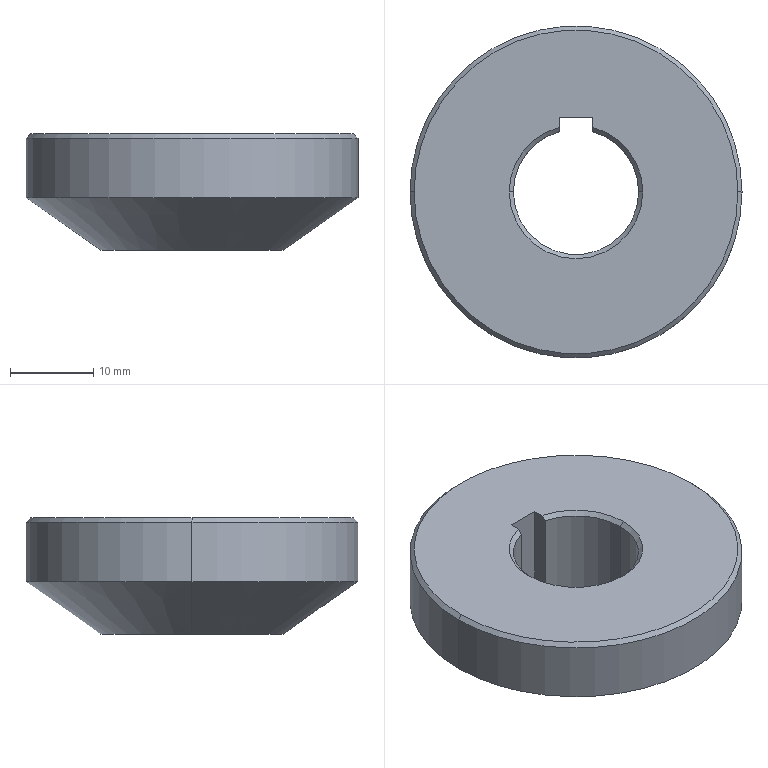Part | STEP file | 10000020570swp000-1 | 1 solid | 20 faces | box 40 x 40 x 14 mm | volume 11944 mm3 | cone 10 | cylinder 5 | plane 5 | commonest cylinder face diameters 15.1 x3 40 x2
STEP:
#1=CARTESIAN_POINT('',(-7.55,0.,-0.5));
#2=VERTEX_POINT('',#1);
#3=CARTESIAN_POINT('',(7.55,0.,-0.5));
#4=VERTEX_POINT('',#3);
#5=CARTESIAN_POINT('',(0.,0.,-0.5));
#6=DIRECTION('',(0.,0.,1.));
#7=DIRECTION('',(1.,0.,0.));
#8=AXIS2_PLACEMENT_3D('',#5,#6,#7);
#9=CIRCLE('',#8,7.55);
#10=EDGE_CURVE('',#2,#4,#9,.T.);
#11=ORIENTED_EDGE('',*,*,#10,.F.);
#12=CARTESIAN_POINT('',(-8.05,0.,0.));
#13=VERTEX_POINT('',#12);
#14=CARTESIAN_POINT('',(-7.55,0.,-0.5));
#15=DIRECTION('',(-0.7071,0.,0.7071));
#16=VECTOR('',#15,1000.);
#17=LINE('',#14,#16);
#18=EDGE_CURVE('',#2,#13,#17,.T.);
#19=ORIENTED_EDGE('',*,*,#18,.T.);
#20=CARTESIAN_POINT('',(8.05,0.,0.));
#21=VERTEX_POINT('',#20);
#22=CARTESIAN_POINT('',(0.,0.,0.));
#23=DIRECTION('',(0.,0.,-1.));
#24=DIRECTION('',(1.,0.,0.));
#25=AXIS2_PLACEMENT_3D('',#22,#23,#24);
#26=CIRCLE('',#25,8.05);
#27=EDGE_CURVE('',#21,#13,#26,.T.);
#28=ORIENTED_EDGE('',*,*,#27,.F.);
#29=CARTESIAN_POINT('',(7.55,0.,-0.5));
#30=DIRECTION('',(0.7071,0.,0.7071));
#31=VECTOR('',#30,1000.);
#32=LINE('',#29,#31);
#33=EDGE_CURVE('',#4,#21,#32,.T.);
#34=ORIENTED_EDGE('',*,*,#33,.F.);
#35=EDGE_LOOP('',(#11,#19,#28,#34));
#36=FACE_OUTER_BOUND('',#35,.T.);
#37=CARTESIAN_POINT('',(0.,0.,-0.5));
#38=DIRECTION('',(0.,0.,1.));
#39=DIRECTION('',(1.,0.,0.));
#40=AXIS2_PLACEMENT_3D('',#37,#38,#39);
#41=CONICAL_SURFACE('',#40,7.55,0.7854);
#42=ADVANCED_FACE('',(#36),#41,.F.);
#43=CARTESIAN_POINT('',(2.,7.28,-0.5));
#44=VERTEX_POINT('',#43);
#45=CARTESIAN_POINT('',(0.,0.,-0.5));
#46=DIRECTION('',(0.,0.,1.));
#47=DIRECTION('',(1.,0.,0.));
#48=AXIS2_PLACEMENT_3D('',#45,#46,#47);
#49=CIRCLE('',#48,7.55);
#50=EDGE_CURVE('',#4,#44,#49,.T.);
#51=ORIENTED_EDGE('',*,*,#50,.F.);
#52=ORIENTED_EDGE('',*,*,#33,.T.);
#53=CARTESIAN_POINT('',(2.,7.798,0.));
#54=VERTEX_POINT('',#53);
#55=CARTESIAN_POINT('',(0.,0.,0.));
#56=DIRECTION('',(0.,0.,-1.));
#57=DIRECTION('',(1.,0.,0.));
#58=AXIS2_PLACEMENT_3D('',#55,#56,#57);
#59=CIRCLE('',#58,8.05);
#60=EDGE_CURVE('',#54,#21,#59,.T.);
#61=ORIENTED_EDGE('',*,*,#60,.F.);
#62=CARTESIAN_POINT('',(2.,7.28,-0.5));
#63=CARTESIAN_POINT('',(2.,7.453,-0.3335));
#64=CARTESIAN_POINT('',(2.,7.625,-0.1669));
#65=CARTESIAN_POINT('',(2.,7.798,0.));
#66=B_SPLINE_CURVE_WITH_KNOTS('',3,(#62,#63,#64,#65),.UNSPECIFIED.,.F.,.F.,(4,4),(0.,0.0007195),.UNSPECIFIED.);
#67=EDGE_CURVE('',#44,#54,#66,.T.);
#68=ORIENTED_EDGE('',*,*,#67,.F.);
#69=EDGE_LOOP('',(#51,#52,#61,#68));
#70=FACE_OUTER_BOUND('',#69,.T.);
#71=CARTESIAN_POINT('',(0.,0.,-0.5));
#72=DIRECTION('',(0.,0.,1.));
#73=DIRECTION('',(1.,0.,0.));
#74=AXIS2_PLACEMENT_3D('',#71,#72,#73);
#75=CONICAL_SURFACE('',#74,7.55,0.7854);
#76=ADVANCED_FACE('',(#70),#75,.F.);
#77=CARTESIAN_POINT('',(7.55,0.,-13.5));
#78=VERTEX_POINT('',#77);
#79=CARTESIAN_POINT('',(-7.55,0.,-13.5));
#80=VERTEX_POINT('',#79);
#81=CARTESIAN_POINT('',(0.,0.,-13.5));
#82=DIRECTION('',(0.,0.,-1.));
#83=DIRECTION('',(1.,0.,0.));
#84=AXIS2_PLACEMENT_3D('',#81,#82,#83);
#85=CIRCLE('',#84,7.55);
#86=EDGE_CURVE('',#78,#80,#85,.T.);
#87=ORIENTED_EDGE('',*,*,#86,.F.);
#88=CARTESIAN_POINT('',(8.05,0.,-14.));
#89=VERTEX_POINT('',#88);
#90=CARTESIAN_POINT('',(8.05,0.,-14.));
#91=DIRECTION('',(0.7071,0.,-0.7071));
#92=VECTOR('',#91,1000.);
#93=LINE('',#90,#92);
#94=EDGE_CURVE('',#78,#89,#93,.T.);
#95=ORIENTED_EDGE('',*,*,#94,.T.);
#96=CARTESIAN_POINT('',(-8.05,0.,-14.));
#97=VERTEX_POINT('',#96);
#98=CARTESIAN_POINT('',(0.,0.,-14.));
#99=DIRECTION('',(0.,0.,1.));
#100=DIRECTION('',(1.,0.,0.));
#101=AXIS2_PLACEMENT_3D('',#98,#99,#100);
#102=CIRCLE('',#101,8.05);
#103=EDGE_CURVE('',#97,#89,#102,.T.);
#104=ORIENTED_EDGE('',*,*,#103,.F.);
#105=CARTESIAN_POINT('',(-8.05,0.,-14.));
#106=DIRECTION('',(-0.7071,0.,-0.7071));
#107=VECTOR('',#106,1000.);
#108=LINE('',#105,#107);
#109=EDGE_CURVE('',#80,#97,#108,.T.);
#110=ORIENTED_EDGE('',*,*,#109,.F.);
#111=EDGE_LOOP('',(#87,#95,#104,#110));
#112=FACE_OUTER_BOUND('',#111,.T.);
#113=CARTESIAN_POINT('',(0.,0.,-14.));
#114=DIRECTION('',(0.,0.,-1.));
#115=DIRECTION('',(-1.,0.,0.));
#116=AXIS2_PLACEMENT_3D('',#113,#114,#115);
#117=CONICAL_SURFACE('',#116,8.05,0.7854);
#118=ADVANCED_FACE('',(#112),#117,.F.);
#119=CARTESIAN_POINT('',(-2.,7.28,-13.5));
#120=VERTEX_POINT('',#119);
#121=CARTESIAN_POINT('',(0.,0.,-13.5));
#122=DIRECTION('',(0.,0.,-1.));
#123=DIRECTION('',(1.,0.,0.));
#124=AXIS2_PLACEMENT_3D('',#121,#122,#123);
#125=CIRCLE('',#124,7.55);
#126=EDGE_CURVE('',#80,#120,#125,.T.);
#127=ORIENTED_EDGE('',*,*,#126,.F.);
#128=ORIENTED_EDGE('',*,*,#109,.T.);
#129=CARTESIAN_POINT('',(-2.,7.798,-14.));
#130=VERTEX_POINT('',#129);
#131=CARTESIAN_POINT('',(0.,0.,-14.));
#132=DIRECTION('',(0.,0.,1.));
#133=DIRECTION('',(1.,0.,0.));
#134=AXIS2_PLACEMENT_3D('',#131,#132,#133);
#135=CIRCLE('',#134,8.05);
#136=EDGE_CURVE('',#130,#97,#135,.T.);
#137=ORIENTED_EDGE('',*,*,#136,.F.);
#138=CARTESIAN_POINT('',(-2.,7.28,-13.5));
#139=CARTESIAN_POINT('',(-2.,7.453,-13.666));
#140=CARTESIAN_POINT('',(-2.,7.625,-13.833));
#141=CARTESIAN_POINT('',(-2.,7.798,-14.));
#142=B_SPLINE_CURVE_WITH_KNOTS('',3,(#138,#139,#140,#141),.UNSPECIFIED.,.F.,.F.,(4,4),(0.,0.0007195),.UNSPECIFIED.);
#143=EDGE_CURVE('',#120,#130,#142,.T.);
#144=ORIENTED_EDGE('',*,*,#143,.F.);
#145=EDGE_LOOP('',(#127,#128,#137,#144));
#146=FACE_OUTER_BOUND('',#145,.T.);
#147=CARTESIAN_POINT('',(0.,0.,-14.));
#148=DIRECTION('',(0.,0.,-1.));
#149=DIRECTION('',(-1.,0.,0.));
#150=AXIS2_PLACEMENT_3D('',#147,#148,#149);
#151=CONICAL_SURFACE('',#150,8.05,0.7854);
#152=ADVANCED_FACE('',(#146),#151,.F.);
#153=CARTESIAN_POINT('',(19.5,0.,0.));
#154=VERTEX_POINT('',#153);
#155=CARTESIAN_POINT('',(-19.5,0.,0.));
#156=VERTEX_POINT('',#155);
#157=CARTESIAN_POINT('',(0.,0.,0.));
#158=DIRECTION('',(0.,0.,1.));
#159=DIRECTION('',(1.,0.,0.));
#160=AXIS2_PLACEMENT_3D('',#157,#158,#159);
#161=CIRCLE('',#160,19.5);
#162=EDGE_CURVE('',#154,#156,#161,.T.);
#163=ORIENTED_EDGE('',*,*,#162,.F.);
#164=CARTESIAN_POINT('',(20.,0.,-0.5));
#165=VERTEX_POINT('',#164);
#166=CARTESIAN_POINT('',(19.5,0.,0.));
#167=DIRECTION('',(0.7071,0.,-0.7071));
#168=VECTOR('',#167,1000.);
#169=LINE('',#166,#168);
#170=EDGE_CURVE('',#154,#165,#169,.T.);
#171=ORIENTED_EDGE('',*,*,#170,.T.);
#172=CARTESIAN_POINT('',(-20.,0.,-0.5));
#173=VERTEX_POINT('',#172);
#174=CARTESIAN_POINT('',(0.,0.,-0.5));
#175=DIRECTION('',(0.,0.,-1.));
#176=DIRECTION('',(1.,0.,0.));
#177=AXIS2_PLACEMENT_3D('',#174,#175,#176);
#178=CIRCLE('',#177,20.);
#179=EDGE_CURVE('',#173,#165,#178,.T.);
#180=ORIENTED_EDGE('',*,*,#179,.F.);
#181=CARTESIAN_POINT('',(-19.5,0.,0.));
#182=DIRECTION('',(-0.7071,0.,-0.7071));
#183=VECTOR('',#182,1000.);
#184=LINE('',#181,#183);
#185=EDGE_CURVE('',#156,#173,#184,.T.);
#186=ORIENTED_EDGE('',*,*,#185,.F.);
#187=EDGE_LOOP('',(#163,#171,#180,#186));
#188=FACE_OUTER_BOUND('',#187,.T.);
#189=CARTESIAN_POINT('',(0.,0.,0.));
#190=DIRECTION('',(0.,0.,-1.));
#191=DIRECTION('',(-1.,0.,0.));
#192=AXIS2_PLACEMENT_3D('',#189,#190,#191);
#193=CONICAL_SURFACE('',#192,19.5,0.7854);
#194=ADVANCED_FACE('',(#188),#193,.T.);
#195=CARTESIAN_POINT('',(11.,0.,-14.));
#196=VERTEX_POINT('',#195);
#197=CARTESIAN_POINT('',(-11.,0.,-14.));
#198=VERTEX_POINT('',#197);
#199=CARTESIAN_POINT('',(0.,0.,-14.));
#200=DIRECTION('',(0.,0.,1.));
#201=DIRECTION('',(1.,0.,0.));
#202=AXIS2_PLACEMENT_3D('',#199,#200,#201);
#203=CIRCLE('',#202,11.);
#204=EDGE_CURVE('',#196,#198,#203,.T.);
#205=ORIENTED_EDGE('',*,*,#204,.T.);
#206=CARTESIAN_POINT('',(-20.,0.,-7.698));
#207=VERTEX_POINT('',#206);
#208=CARTESIAN_POINT('',(-11.,0.,-14.));
#209=DIRECTION('',(-0.8192,0.,0.5736));
#210=VECTOR('',#209,1000.);
#211=LINE('',#208,#210);
#212=EDGE_CURVE('',#198,#207,#211,.T.);
#213=ORIENTED_EDGE('',*,*,#212,.T.);
#214=CARTESIAN_POINT('',(20.,0.,-7.698));
#215=VERTEX_POINT('',#214);
#216=CARTESIAN_POINT('',(0.,0.,-7.698));
#217=DIRECTION('',(0.,0.,1.));
#218=DIRECTION('',(1.,0.,0.));
#219=AXIS2_PLACEMENT_3D('',#216,#217,#218);
#220=CIRCLE('',#219,20.);
#221=EDGE_CURVE('',#215,#207,#220,.T.);
#222=ORIENTED_EDGE('',*,*,#221,.F.);
#223=CARTESIAN_POINT('',(11.,0.,-14.));
#224=DIRECTION('',(0.8192,0.,0.5736));
#225=VECTOR('',#224,1000.);
#226=LINE('',#223,#225);
#227=EDGE_CURVE('',#196,#215,#226,.T.);
#228=ORIENTED_EDGE('',*,*,#227,.F.);
#229=EDGE_LOOP('',(#205,#213,#222,#228));
#230=FACE_OUTER_BOUND('',#229,.T.);
#231=CARTESIAN_POINT('',(0.,0.,-14.));
#232=DIRECTION('',(0.,0.,1.));
#233=DIRECTION('',(1.,0.,0.));
#234=AXIS2_PLACEMENT_3D('',#231,#232,#233);
#235=CONICAL_SURFACE('',#234,11.,0.9599);
#236=ADVANCED_FACE('',(#230),#235,.T.);
#237=ORIENTED_EDGE('',*,*,#86,.T.);
#238=CARTESIAN_POINT('',(-7.55,0.,-14.));
#239=DIRECTION('',(0.,0.,1.));
#240=VECTOR('',#239,1000.);
#241=LINE('',#238,#240);
#242=EDGE_CURVE('',#80,#2,#241,.T.);
#243=ORIENTED_EDGE('',*,*,#242,.T.);
#244=ORIENTED_EDGE('',*,*,#10,.T.);
#245=CARTESIAN_POINT('',(7.55,0.,-14.));
#246=DIRECTION('',(0.,0.,1.));
#247=VECTOR('',#246,1000.);
#248=LINE('',#245,#247);
#249=EDGE_CURVE('',#78,#4,#248,.T.);
#250=ORIENTED_EDGE('',*,*,#249,.F.);
#251=EDGE_LOOP('',(#237,#243,#244,#250));
#252=FACE_OUTER_BOUND('',#251,.T.);
#253=CARTESIAN_POINT('',(0.,0.,-14.));
#254=DIRECTION('',(0.,0.,1.));
#255=DIRECTION('',(1.,0.,0.));
#256=AXIS2_PLACEMENT_3D('',#253,#254,#255);
#257=CYLINDRICAL_SURFACE('',#256,7.55);
#258=ADVANCED_FACE('',(#252),#257,.F.);
#259=CARTESIAN_POINT('',(2.,7.28,-13.5));
#260=VERTEX_POINT('',#259);
#261=CARTESIAN_POINT('',(0.,0.,-13.5));
#262=DIRECTION('',(0.,0.,-1.));
#263=DIRECTION('',(1.,0.,0.));
#264=AXIS2_PLACEMENT_3D('',#261,#262,#263);
#265=CIRCLE('',#264,7.55);
#266=EDGE_CURVE('',#260,#78,#265,.T.);
#267=ORIENTED_EDGE('',*,*,#266,.T.);
#268=ORIENTED_EDGE('',*,*,#249,.T.);
#269=ORIENTED_EDGE('',*,*,#50,.T.);
#270=CARTESIAN_POINT('',(2.,7.28,-14.));
#271=DIRECTION('',(0.,0.,-1.));
#272=VECTOR('',#271,1000.);
#273=LINE('',#270,#272);
#274=EDGE_CURVE('',#44,#260,#273,.T.);
#275=ORIENTED_EDGE('',*,*,#274,.T.);
#276=EDGE_LOOP('',(#267,#268,#269,#275));
#277=FACE_OUTER_BOUND('',#276,.T.);
#278=CARTESIAN_POINT('',(0.,0.,-14.));
#279=DIRECTION('',(0.,0.,1.));
#280=DIRECTION('',(1.,0.,0.));
#281=AXIS2_PLACEMENT_3D('',#278,#279,#280);
#282=CYLINDRICAL_SURFACE('',#281,7.55);
#283=ADVANCED_FACE('',(#277),#282,.F.);
#284=ORIENTED_EDGE('',*,*,#221,.T.);
#285=CARTESIAN_POINT('',(-20.,0.,-14.));
#286=DIRECTION('',(0.,0.,1.));
#287=VECTOR('',#286,1000.);
#288=LINE('',#285,#287);
#289=EDGE_CURVE('',#207,#173,#288,.T.);
#290=ORIENTED_EDGE('',*,*,#289,.T.);
#291=ORIENTED_EDGE('',*,*,#179,.T.);
#292=CARTESIAN_POINT('',(20.,0.,-14.));
#293=DIRECTION('',(0.,0.,1.));
#294=VECTOR('',#293,1000.);
#295=LINE('',#292,#294);
#296=EDGE_CURVE('',#215,#165,#295,.T.);
#297=ORIENTED_EDGE('',*,*,#296,.F.);
#298=EDGE_LOOP('',(#284,#290,#291,#297));
#299=FACE_OUTER_BOUND('',#298,.T.);
#300=CARTESIAN_POINT('',(0.,0.,-14.));
#301=DIRECTION('',(0.,0.,1.));
#302=DIRECTION('',(1.,0.,0.));
#303=AXIS2_PLACEMENT_3D('',#300,#301,#302);
#304=CYLINDRICAL_SURFACE('',#303,20.);
#305=ADVANCED_FACE('',(#299),#304,.T.);
#306=CARTESIAN_POINT('',(-2.,9.,-14.));
#307=VERTEX_POINT('',#306);
#308=CARTESIAN_POINT('',(-2.,9.,-14.));
#309=DIRECTION('',(0.,-1.,0.));
#310=VECTOR('',#309,1000.);
#311=LINE('',#308,#310);
#312=EDGE_CURVE('',#307,#130,#311,.T.);
#313=ORIENTED_EDGE('',*,*,#312,.T.);
#314=ORIENTED_EDGE('',*,*,#136,.T.);
#315=ORIENTED_EDGE('',*,*,#103,.T.);
#316=CARTESIAN_POINT('',(2.,7.798,-14.));
#317=VERTEX_POINT('',#316);
#318=CARTESIAN_POINT('',(0.,0.,-14.));
#319=DIRECTION('',(0.,0.,1.));
#320=DIRECTION('',(1.,0.,0.));
#321=AXIS2_PLACEMENT_3D('',#318,#319,#320);
#322=CIRCLE('',#321,8.05);
#323=EDGE_CURVE('',#89,#317,#322,.T.);
#324=ORIENTED_EDGE('',*,*,#323,.T.);
#325=CARTESIAN_POINT('',(2.,9.,-14.));
#326=VERTEX_POINT('',#325);
#327=CARTESIAN_POINT('',(2.,9.,-14.));
#328=DIRECTION('',(0.,1.,0.));
#329=VECTOR('',#328,1000.);
#330=LINE('',#327,#329);
#331=EDGE_CURVE('',#317,#326,#330,.T.);
#332=ORIENTED_EDGE('',*,*,#331,.T.);
#333=CARTESIAN_POINT('',(-2.,9.,-14.));
#334=DIRECTION('',(-1.,0.,0.));
#335=VECTOR('',#334,1000.);
#336=LINE('',#333,#335);
#337=EDGE_CURVE('',#326,#307,#336,.T.);
#338=ORIENTED_EDGE('',*,*,#337,.T.);
#339=EDGE_LOOP('',(#313,#314,#315,#324,#332,#338));
#340=FACE_BOUND('',#339,.T.);
#341=ORIENTED_EDGE('',*,*,#204,.F.);
#342=CARTESIAN_POINT('',(0.,0.,-14.));
#343=DIRECTION('',(0.,0.,1.));
#344=DIRECTION('',(1.,0.,0.));
#345=AXIS2_PLACEMENT_3D('',#342,#343,#344);
#346=CIRCLE('',#345,11.);
#347=EDGE_CURVE('',#198,#196,#346,.T.);
#348=ORIENTED_EDGE('',*,*,#347,.F.);
#349=EDGE_LOOP('',(#341,#348));
#350=FACE_OUTER_BOUND('',#349,.T.);
#351=CARTESIAN_POINT('',(0.,0.,-14.));
#352=DIRECTION('',(0.,0.,1.));
#353=DIRECTION('',(1.,0.,0.));
#354=AXIS2_PLACEMENT_3D('',#351,#352,#353);
#355=PLANE('',#354);
#356=ADVANCED_FACE('',(#340,#350),#355,.F.);
#357=ORIENTED_EDGE('',*,*,#289,.F.);
#358=CARTESIAN_POINT('',(0.,0.,-7.698));
#359=DIRECTION('',(0.,0.,1.));
#360=DIRECTION('',(1.,0.,0.));
#361=AXIS2_PLACEMENT_3D('',#358,#359,#360);
#362=CIRCLE('',#361,20.);
#363=EDGE_CURVE('',#207,#215,#362,.T.);
#364=ORIENTED_EDGE('',*,*,#363,.T.);
#365=ORIENTED_EDGE('',*,*,#296,.T.);
#366=CARTESIAN_POINT('',(0.,0.,-0.5));
#367=DIRECTION('',(0.,0.,-1.));
#368=DIRECTION('',(1.,0.,0.));
#369=AXIS2_PLACEMENT_3D('',#366,#367,#368);
#370=CIRCLE('',#369,20.);
#371=EDGE_CURVE('',#165,#173,#370,.T.);
#372=ORIENTED_EDGE('',*,*,#371,.T.);
#373=EDGE_LOOP('',(#357,#364,#365,#372));
#374=FACE_OUTER_BOUND('',#373,.T.);
#375=CARTESIAN_POINT('',(0.,0.,-14.));
#376=DIRECTION('',(0.,0.,1.));
#377=DIRECTION('',(1.,0.,0.));
#378=AXIS2_PLACEMENT_3D('',#375,#376,#377);
#379=CYLINDRICAL_SURFACE('',#378,20.);
#380=ADVANCED_FACE('',(#374),#379,.T.);
#381=CARTESIAN_POINT('',(0.,0.,0.));
#382=DIRECTION('',(0.,0.,1.));
#383=DIRECTION('',(1.,0.,0.));
#384=AXIS2_PLACEMENT_3D('',#381,#382,#383);
#385=CIRCLE('',#384,19.5);
#386=EDGE_CURVE('',#156,#154,#385,.T.);
#387=ORIENTED_EDGE('',*,*,#386,.T.);
#388=ORIENTED_EDGE('',*,*,#162,.T.);
#389=EDGE_LOOP('',(#387,#388));
#390=FACE_OUTER_BOUND('',#389,.T.);
#391=CARTESIAN_POINT('',(2.,9.,0.));
#392=VERTEX_POINT('',#391);
#393=CARTESIAN_POINT('',(2.,9.,0.));
#394=DIRECTION('',(0.,1.,0.));
#395=VECTOR('',#394,1000.);
#396=LINE('',#393,#395);
#397=EDGE_CURVE('',#54,#392,#396,.T.);
#398=ORIENTED_EDGE('',*,*,#397,.F.);
#399=ORIENTED_EDGE('',*,*,#60,.T.);
#400=ORIENTED_EDGE('',*,*,#27,.T.);
#401=CARTESIAN_POINT('',(-2.,7.798,0.));
#402=VERTEX_POINT('',#401);
#403=CARTESIAN_POINT('',(0.,0.,0.));
#404=DIRECTION('',(0.,0.,-1.));
#405=DIRECTION('',(1.,0.,0.));
#406=AXIS2_PLACEMENT_3D('',#403,#404,#405);
#407=CIRCLE('',#406,8.05);
#408=EDGE_CURVE('',#13,#402,#407,.T.);
#409=ORIENTED_EDGE('',*,*,#408,.T.);
#410=CARTESIAN_POINT('',(-2.,9.,0.));
#411=VERTEX_POINT('',#410);
#412=CARTESIAN_POINT('',(-2.,9.,0.));
#413=DIRECTION('',(0.,-1.,0.));
#414=VECTOR('',#413,1000.);
#415=LINE('',#412,#414);
#416=EDGE_CURVE('',#411,#402,#415,.T.);
#417=ORIENTED_EDGE('',*,*,#416,.F.);
#418=CARTESIAN_POINT('',(-2.,9.,0.));
#419=DIRECTION('',(-1.,0.,0.));
#420=VECTOR('',#419,1000.);
#421=LINE('',#418,#420);
#422=EDGE_CURVE('',#392,#411,#421,.T.);
#423=ORIENTED_EDGE('',*,*,#422,.F.);
#424=EDGE_LOOP('',(#398,#399,#400,#409,#417,#423));
#425=FACE_BOUND('',#424,.T.);
#426=CARTESIAN_POINT('',(0.,0.,0.));
#427=DIRECTION('',(0.,0.,1.));
#428=DIRECTION('',(1.,0.,0.));
#429=AXIS2_PLACEMENT_3D('',#426,#427,#428);
#430=PLANE('',#429);
#431=ADVANCED_FACE('',(#390,#425),#430,.T.);
#432=ORIENTED_EDGE('',*,*,#242,.F.);
#433=ORIENTED_EDGE('',*,*,#126,.T.);
#434=CARTESIAN_POINT('',(-2.,7.28,-0.5));
#435=VERTEX_POINT('',#434);
#436=CARTESIAN_POINT('',(-2.,7.28,-14.));
#437=DIRECTION('',(0.,0.,1.));
#438=VECTOR('',#437,1000.);
#439=LINE('',#436,#438);
#440=EDGE_CURVE('',#120,#435,#439,.T.);
#441=ORIENTED_EDGE('',*,*,#440,.T.);
#442=CARTESIAN_POINT('',(0.,0.,-0.5));
#443=DIRECTION('',(0.,0.,1.));
#444=DIRECTION('',(1.,0.,0.));
#445=AXIS2_PLACEMENT_3D('',#442,#443,#444);
#446=CIRCLE('',#445,7.55);
#447=EDGE_CURVE('',#435,#2,#446,.T.);
#448=ORIENTED_EDGE('',*,*,#447,.T.);
#449=EDGE_LOOP('',(#432,#433,#441,#448));
#450=FACE_OUTER_BOUND('',#449,.T.);
#451=CARTESIAN_POINT('',(0.,0.,-14.));
#452=DIRECTION('',(0.,0.,1.));
#453=DIRECTION('',(1.,0.,0.));
#454=AXIS2_PLACEMENT_3D('',#451,#452,#453);
#455=CYLINDRICAL_SURFACE('',#454,7.55);
#456=ADVANCED_FACE('',(#450),#455,.F.);
#457=ORIENTED_EDGE('',*,*,#440,.F.);
#458=ORIENTED_EDGE('',*,*,#143,.T.);
#459=ORIENTED_EDGE('',*,*,#312,.F.);
#460=CARTESIAN_POINT('',(-2.,9.,-14.));
#461=DIRECTION('',(0.,0.,1.));
#462=VECTOR('',#461,1000.);
#463=LINE('',#460,#462);
#464=EDGE_CURVE('',#307,#411,#463,.T.);
#465=ORIENTED_EDGE('',*,*,#464,.T.);
#466=ORIENTED_EDGE('',*,*,#416,.T.);
#467=CARTESIAN_POINT('',(-2.,7.798,0.));
#468=CARTESIAN_POINT('',(-2.,7.625,-0.1669));
#469=CARTESIAN_POINT('',(-2.,7.453,-0.3335));
#470=CARTESIAN_POINT('',(-2.,7.28,-0.5));
#471=B_SPLINE_CURVE_WITH_KNOTS('',3,(#467,#468,#469,#470),.UNSPECIFIED.,.F.,.F.,(4,4),(0.,0.0007195),.UNSPECIFIED.);
#472=EDGE_CURVE('',#402,#435,#471,.T.);
#473=ORIENTED_EDGE('',*,*,#472,.T.);
#474=EDGE_LOOP('',(#457,#458,#459,#465,#466,#473));
#475=FACE_OUTER_BOUND('',#474,.T.);
#476=CARTESIAN_POINT('',(-2.,9.,-14.));
#477=DIRECTION('',(-1.,0.,0.));
#478=DIRECTION('',(0.,-1.,0.));
#479=AXIS2_PLACEMENT_3D('',#476,#477,#478);
#480=PLANE('',#479);
#481=ADVANCED_FACE('',(#475),#480,.F.);
#482=ORIENTED_EDGE('',*,*,#331,.F.);
#483=CARTESIAN_POINT('',(2.,7.798,-14.));
#484=CARTESIAN_POINT('',(2.,7.625,-13.833));
#485=CARTESIAN_POINT('',(2.,7.453,-13.666));
#486=CARTESIAN_POINT('',(2.,7.28,-13.5));
#487=B_SPLINE_CURVE_WITH_KNOTS('',3,(#483,#484,#485,#486),.UNSPECIFIED.,.F.,.F.,(4,4),(0.,0.0007195),.UNSPECIFIED.);
#488=EDGE_CURVE('',#317,#260,#487,.T.);
#489=ORIENTED_EDGE('',*,*,#488,.T.);
#490=ORIENTED_EDGE('',*,*,#274,.F.);
#491=ORIENTED_EDGE('',*,*,#67,.T.);
#492=ORIENTED_EDGE('',*,*,#397,.T.);
#493=CARTESIAN_POINT('',(2.,9.,-14.));
#494=DIRECTION('',(0.,0.,1.));
#495=VECTOR('',#494,1000.);
#496=LINE('',#493,#495);
#497=EDGE_CURVE('',#326,#392,#496,.T.);
#498=ORIENTED_EDGE('',*,*,#497,.F.);
#499=EDGE_LOOP('',(#482,#489,#490,#491,#492,#498));
#500=FACE_OUTER_BOUND('',#499,.T.);
#501=CARTESIAN_POINT('',(2.,9.,-14.));
#502=DIRECTION('',(1.,0.,0.));
#503=DIRECTION('',(0.,1.,0.));
#504=AXIS2_PLACEMENT_3D('',#501,#502,#503);
#505=PLANE('',#504);
#506=ADVANCED_FACE('',(#500),#505,.F.);
#507=ORIENTED_EDGE('',*,*,#422,.T.);
#508=ORIENTED_EDGE('',*,*,#464,.F.);
#509=ORIENTED_EDGE('',*,*,#337,.F.);
#510=ORIENTED_EDGE('',*,*,#497,.T.);
#511=EDGE_LOOP('',(#507,#508,#509,#510));
#512=FACE_OUTER_BOUND('',#511,.T.);
#513=CARTESIAN_POINT('',(-2.,9.,-14.));
#514=DIRECTION('',(0.,1.,0.));
#515=DIRECTION('',(0.,0.,1.));
#516=AXIS2_PLACEMENT_3D('',#513,#514,#515);
#517=PLANE('',#516);
#518=ADVANCED_FACE('',(#512),#517,.F.);
#519=ORIENTED_EDGE('',*,*,#212,.F.);
#520=ORIENTED_EDGE('',*,*,#347,.T.);
#521=ORIENTED_EDGE('',*,*,#227,.T.);
#522=ORIENTED_EDGE('',*,*,#363,.F.);
#523=EDGE_LOOP('',(#519,#520,#521,#522));
#524=FACE_OUTER_BOUND('',#523,.T.);
#525=CARTESIAN_POINT('',(0.,0.,-14.));
#526=DIRECTION('',(0.,0.,1.));
#527=DIRECTION('',(1.,0.,0.));
#528=AXIS2_PLACEMENT_3D('',#525,#526,#527);
#529=CONICAL_SURFACE('',#528,11.,0.9599);
#530=ADVANCED_FACE('',(#524),#529,.T.);
#531=ORIENTED_EDGE('',*,*,#170,.F.);
#532=ORIENTED_EDGE('',*,*,#386,.F.);
#533=ORIENTED_EDGE('',*,*,#185,.T.);
#534=ORIENTED_EDGE('',*,*,#371,.F.);
#535=EDGE_LOOP('',(#531,#532,#533,#534));
#536=FACE_OUTER_BOUND('',#535,.T.);
#537=CARTESIAN_POINT('',(0.,0.,0.));
#538=DIRECTION('',(0.,0.,-1.));
#539=DIRECTION('',(-1.,0.,0.));
#540=AXIS2_PLACEMENT_3D('',#537,#538,#539);
#541=CONICAL_SURFACE('',#540,19.5,0.7854);
#542=ADVANCED_FACE('',(#536),#541,.T.);
#543=ORIENTED_EDGE('',*,*,#94,.F.);
#544=ORIENTED_EDGE('',*,*,#266,.F.);
#545=ORIENTED_EDGE('',*,*,#488,.F.);
#546=ORIENTED_EDGE('',*,*,#323,.F.);
#547=EDGE_LOOP('',(#543,#544,#545,#546));
#548=FACE_OUTER_BOUND('',#547,.T.);
#549=CARTESIAN_POINT('',(0.,0.,-14.));
#550=DIRECTION('',(0.,0.,-1.));
#551=DIRECTION('',(-1.,0.,0.));
#552=AXIS2_PLACEMENT_3D('',#549,#550,#551);
#553=CONICAL_SURFACE('',#552,8.05,0.7854);
#554=ADVANCED_FACE('',(#548),#553,.F.);
#555=ORIENTED_EDGE('',*,*,#18,.F.);
#556=ORIENTED_EDGE('',*,*,#447,.F.);
#557=ORIENTED_EDGE('',*,*,#472,.F.);
#558=ORIENTED_EDGE('',*,*,#408,.F.);
#559=EDGE_LOOP('',(#555,#556,#557,#558));
#560=FACE_OUTER_BOUND('',#559,.T.);
#561=CARTESIAN_POINT('',(0.,0.,-0.5));
#562=DIRECTION('',(0.,0.,1.));
#563=DIRECTION('',(1.,0.,0.));
#564=AXIS2_PLACEMENT_3D('',#561,#562,#563);
#565=CONICAL_SURFACE('',#564,7.55,0.7854);
#566=ADVANCED_FACE('',(#560),#565,.F.);
#567=CLOSED_SHELL('',(#42,#76,#118,#152,#194,#236,#258,#283,#305,#356,#380,#431,#456,#481,#506,#518,#530,#542,#554,#566));
#568=MANIFOLD_SOLID_BREP('',#567);
#569=CARTESIAN_POINT('',(0.,0.,0.));
#570=DIRECTION('',(0.,0.,1.));
#571=DIRECTION('',(1.,0.,0.));
#572=AXIS2_PLACEMENT_3D('',#569,#570,#571);
#573=(LENGTH_UNIT()NAMED_UNIT(*)SI_UNIT(.MILLI.,.METRE.));
#574=UNCERTAINTY_MEASURE_WITH_UNIT(LENGTH_MEASURE(0.00001),#573,'','');
#575=(NAMED_UNIT(*)PLANE_ANGLE_UNIT()SI_UNIT($,.RADIAN.));
#576=(NAMED_UNIT(*)SI_UNIT($,.STERADIAN.)SOLID_ANGLE_UNIT());
#577=(GEOMETRIC_REPRESENTATION_CONTEXT(3)GLOBAL_UNCERTAINTY_ASSIGNED_CONTEXT((#574))GLOBAL_UNIT_ASSIGNED_CONTEXT((#573,#575,#576))REPRESENTATION_CONTEXT('',''));
#578=ADVANCED_BREP_SHAPE_REPRESENTATION('',(#568,#572),#577);